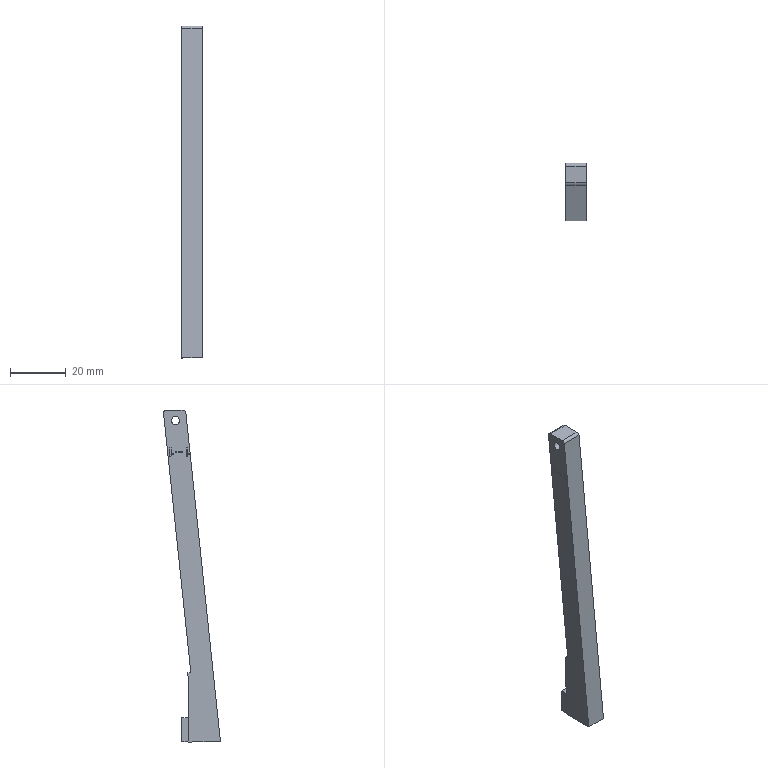Part | STEP file | solid 84 | 1 solid | 35 faces | box 7.5 x 20.479 x 119.36 mm | volume 7713 mm3 | plane 28 | other 4 | cylinder 3 | commonest cylinder face diameters 2 x2 3 x1